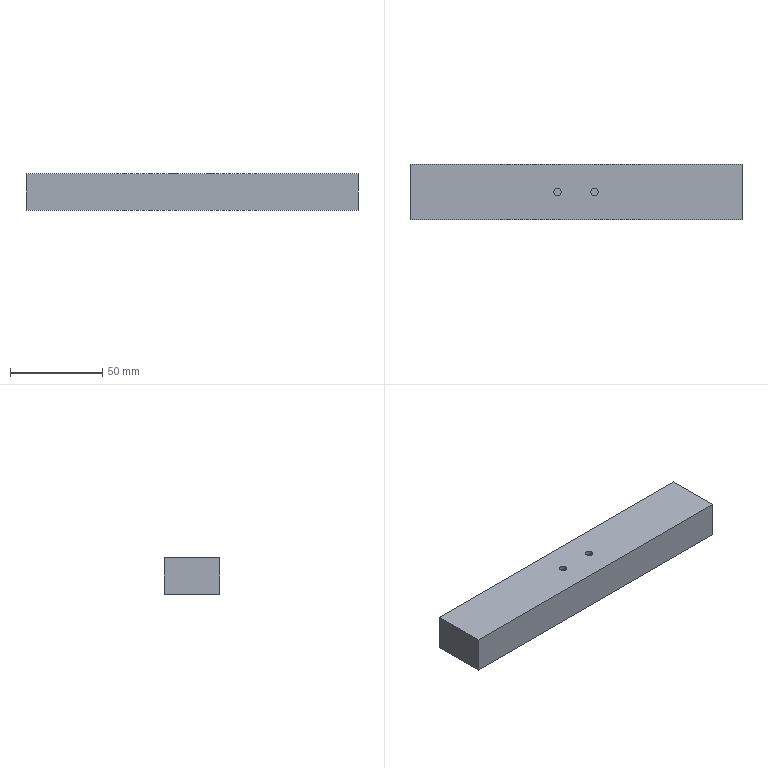Part | SolidWorks | features Extrusion 1, ICE 1 | 1 solid | 12 faces | box 180 x 30 x 20 mm | volume 107950 mm3 | plane 8 | cylinder 4 | commonest cylinder face diameters 4 x4
STEP:
#1=CARTESIAN_POINT('',(-12.,0.,18.));
#2=VERTEX_POINT('',#1);
#3=CARTESIAN_POINT('',(-8.,0.,18.));
#4=VERTEX_POINT('',#3);
#5=CARTESIAN_POINT('',(-10.,0.,18.));
#6=DIRECTION('',(0.,0.,1.));
#7=DIRECTION('',(1.,0.,0.));
#8=AXIS2_PLACEMENT_3D('',#5,#6,#7);
#9=CIRCLE('',#8,2.);
#10=EDGE_CURVE('',#2,#4,#9,.T.);
#11=ORIENTED_EDGE('',*,*,#10,.F.);
#12=CARTESIAN_POINT('',(-12.,0.,20.));
#13=VERTEX_POINT('',#12);
#14=CARTESIAN_POINT('',(-12.,0.,18.));
#15=DIRECTION('',(0.,0.,1.));
#16=VECTOR('',#15,1000.);
#17=LINE('',#14,#16);
#18=EDGE_CURVE('',#2,#13,#17,.T.);
#19=ORIENTED_EDGE('',*,*,#18,.T.);
#20=CARTESIAN_POINT('',(-8.,0.,20.));
#21=VERTEX_POINT('',#20);
#22=CARTESIAN_POINT('',(-10.,0.,20.));
#23=DIRECTION('',(0.,0.,1.));
#24=DIRECTION('',(1.,0.,0.));
#25=AXIS2_PLACEMENT_3D('',#22,#23,#24);
#26=CIRCLE('',#25,2.);
#27=EDGE_CURVE('',#13,#21,#26,.T.);
#28=ORIENTED_EDGE('',*,*,#27,.T.);
#29=CARTESIAN_POINT('',(-8.,0.,18.));
#30=DIRECTION('',(0.,0.,1.));
#31=VECTOR('',#30,1000.);
#32=LINE('',#29,#31);
#33=EDGE_CURVE('',#4,#21,#32,.T.);
#34=ORIENTED_EDGE('',*,*,#33,.F.);
#35=EDGE_LOOP('',(#11,#19,#28,#34));
#36=FACE_OUTER_BOUND('',#35,.T.);
#37=CARTESIAN_POINT('',(-10.,0.,18.));
#38=DIRECTION('',(0.,0.,1.));
#39=DIRECTION('',(1.,0.,0.));
#40=AXIS2_PLACEMENT_3D('',#37,#38,#39);
#41=CYLINDRICAL_SURFACE('',#40,2.);
#42=ADVANCED_FACE('',(#36),#41,.F.);
#43=CARTESIAN_POINT('',(8.,0.,18.));
#44=VERTEX_POINT('',#43);
#45=CARTESIAN_POINT('',(12.,0.,18.));
#46=VERTEX_POINT('',#45);
#47=CARTESIAN_POINT('',(10.,0.,18.));
#48=DIRECTION('',(0.,0.,1.));
#49=DIRECTION('',(1.,0.,0.));
#50=AXIS2_PLACEMENT_3D('',#47,#48,#49);
#51=CIRCLE('',#50,2.);
#52=EDGE_CURVE('',#44,#46,#51,.T.);
#53=ORIENTED_EDGE('',*,*,#52,.F.);
#54=CARTESIAN_POINT('',(8.,0.,20.));
#55=VERTEX_POINT('',#54);
#56=CARTESIAN_POINT('',(8.,0.,18.));
#57=DIRECTION('',(0.,0.,1.));
#58=VECTOR('',#57,1000.);
#59=LINE('',#56,#58);
#60=EDGE_CURVE('',#44,#55,#59,.T.);
#61=ORIENTED_EDGE('',*,*,#60,.T.);
#62=CARTESIAN_POINT('',(12.,0.,20.));
#63=VERTEX_POINT('',#62);
#64=CARTESIAN_POINT('',(10.,0.,20.));
#65=DIRECTION('',(0.,0.,1.));
#66=DIRECTION('',(1.,0.,0.));
#67=AXIS2_PLACEMENT_3D('',#64,#65,#66);
#68=CIRCLE('',#67,2.);
#69=EDGE_CURVE('',#55,#63,#68,.T.);
#70=ORIENTED_EDGE('',*,*,#69,.T.);
#71=CARTESIAN_POINT('',(12.,0.,18.));
#72=DIRECTION('',(0.,0.,1.));
#73=VECTOR('',#72,1000.);
#74=LINE('',#71,#73);
#75=EDGE_CURVE('',#46,#63,#74,.T.);
#76=ORIENTED_EDGE('',*,*,#75,.F.);
#77=EDGE_LOOP('',(#53,#61,#70,#76));
#78=FACE_OUTER_BOUND('',#77,.T.);
#79=CARTESIAN_POINT('',(10.,0.,18.));
#80=DIRECTION('',(0.,0.,1.));
#81=DIRECTION('',(1.,0.,0.));
#82=AXIS2_PLACEMENT_3D('',#79,#80,#81);
#83=CYLINDRICAL_SURFACE('',#82,2.);
#84=ADVANCED_FACE('',(#78),#83,.F.);
#85=CARTESIAN_POINT('',(-90.,15.,0.));
#86=VERTEX_POINT('',#85);
#87=CARTESIAN_POINT('',(-90.,-15.,0.));
#88=VERTEX_POINT('',#87);
#89=CARTESIAN_POINT('',(-90.,-15.,0.));
#90=DIRECTION('',(0.,-1.,0.));
#91=VECTOR('',#90,1000.);
#92=LINE('',#89,#91);
#93=EDGE_CURVE('',#86,#88,#92,.T.);
#94=ORIENTED_EDGE('',*,*,#93,.T.);
#95=CARTESIAN_POINT('',(-90.,-15.,20.));
#96=VERTEX_POINT('',#95);
#97=CARTESIAN_POINT('',(-90.,-15.,20.));
#98=DIRECTION('',(0.,0.,-1.));
#99=VECTOR('',#98,1000.);
#100=LINE('',#97,#99);
#101=EDGE_CURVE('',#96,#88,#100,.T.);
#102=ORIENTED_EDGE('',*,*,#101,.F.);
#103=CARTESIAN_POINT('',(-90.,15.,20.));
#104=VERTEX_POINT('',#103);
#105=CARTESIAN_POINT('',(-90.,-15.,20.));
#106=DIRECTION('',(0.,-1.,0.));
#107=VECTOR('',#106,1000.);
#108=LINE('',#105,#107);
#109=EDGE_CURVE('',#104,#96,#108,.T.);
#110=ORIENTED_EDGE('',*,*,#109,.F.);
#111=CARTESIAN_POINT('',(-90.,15.,20.));
#112=DIRECTION('',(0.,0.,-1.));
#113=VECTOR('',#112,1000.);
#114=LINE('',#111,#113);
#115=EDGE_CURVE('',#104,#86,#114,.T.);
#116=ORIENTED_EDGE('',*,*,#115,.T.);
#117=EDGE_LOOP('',(#94,#102,#110,#116));
#118=FACE_OUTER_BOUND('',#117,.T.);
#119=CARTESIAN_POINT('',(-90.,-15.,20.));
#120=DIRECTION('',(1.,0.,0.));
#121=DIRECTION('',(0.,0.,-1.));
#122=AXIS2_PLACEMENT_3D('',#119,#120,#121);
#123=PLANE('',#122);
#124=ADVANCED_FACE('',(#118),#123,.F.);
#125=CARTESIAN_POINT('',(90.,-15.,0.));
#126=VERTEX_POINT('',#125);
#127=CARTESIAN_POINT('',(90.,-15.,0.));
#128=DIRECTION('',(1.,0.,0.));
#129=VECTOR('',#128,1000.);
#130=LINE('',#127,#129);
#131=EDGE_CURVE('',#88,#126,#130,.T.);
#132=ORIENTED_EDGE('',*,*,#131,.T.);
#133=CARTESIAN_POINT('',(90.,-15.,20.));
#134=VERTEX_POINT('',#133);
#135=CARTESIAN_POINT('',(90.,-15.,20.));
#136=DIRECTION('',(0.,0.,-1.));
#137=VECTOR('',#136,1000.);
#138=LINE('',#135,#137);
#139=EDGE_CURVE('',#134,#126,#138,.T.);
#140=ORIENTED_EDGE('',*,*,#139,.F.);
#141=CARTESIAN_POINT('',(90.,-15.,20.));
#142=DIRECTION('',(1.,0.,0.));
#143=VECTOR('',#142,1000.);
#144=LINE('',#141,#143);
#145=EDGE_CURVE('',#96,#134,#144,.T.);
#146=ORIENTED_EDGE('',*,*,#145,.F.);
#147=ORIENTED_EDGE('',*,*,#101,.T.);
#148=EDGE_LOOP('',(#132,#140,#146,#147));
#149=FACE_OUTER_BOUND('',#148,.T.);
#150=CARTESIAN_POINT('',(90.,-15.,20.));
#151=DIRECTION('',(0.,1.,0.));
#152=DIRECTION('',(-1.,0.,0.));
#153=AXIS2_PLACEMENT_3D('',#150,#151,#152);
#154=PLANE('',#153);
#155=ADVANCED_FACE('',(#149),#154,.F.);
#156=CARTESIAN_POINT('',(90.,15.,0.));
#157=VERTEX_POINT('',#156);
#158=CARTESIAN_POINT('',(90.,-15.,0.));
#159=DIRECTION('',(0.,1.,0.));
#160=VECTOR('',#159,1000.);
#161=LINE('',#158,#160);
#162=EDGE_CURVE('',#126,#157,#161,.T.);
#163=ORIENTED_EDGE('',*,*,#162,.T.);
#164=CARTESIAN_POINT('',(90.,15.,20.));
#165=VERTEX_POINT('',#164);
#166=CARTESIAN_POINT('',(90.,15.,20.));
#167=DIRECTION('',(0.,0.,-1.));
#168=VECTOR('',#167,1000.);
#169=LINE('',#166,#168);
#170=EDGE_CURVE('',#165,#157,#169,.T.);
#171=ORIENTED_EDGE('',*,*,#170,.F.);
#172=CARTESIAN_POINT('',(90.,-15.,20.));
#173=DIRECTION('',(0.,1.,0.));
#174=VECTOR('',#173,1000.);
#175=LINE('',#172,#174);
#176=EDGE_CURVE('',#134,#165,#175,.T.);
#177=ORIENTED_EDGE('',*,*,#176,.F.);
#178=ORIENTED_EDGE('',*,*,#139,.T.);
#179=EDGE_LOOP('',(#163,#171,#177,#178));
#180=FACE_OUTER_BOUND('',#179,.T.);
#181=CARTESIAN_POINT('',(90.,-15.,20.));
#182=DIRECTION('',(-1.,0.,0.));
#183=DIRECTION('',(0.,0.,1.));
#184=AXIS2_PLACEMENT_3D('',#181,#182,#183);
#185=PLANE('',#184);
#186=ADVANCED_FACE('',(#180),#185,.F.);
#187=CARTESIAN_POINT('',(90.,15.,0.));
#188=DIRECTION('',(-1.,0.,0.));
#189=VECTOR('',#188,1000.);
#190=LINE('',#187,#189);
#191=EDGE_CURVE('',#157,#86,#190,.T.);
#192=ORIENTED_EDGE('',*,*,#191,.T.);
#193=ORIENTED_EDGE('',*,*,#115,.F.);
#194=CARTESIAN_POINT('',(90.,15.,20.));
#195=DIRECTION('',(-1.,0.,0.));
#196=VECTOR('',#195,1000.);
#197=LINE('',#194,#196);
#198=EDGE_CURVE('',#165,#104,#197,.T.);
#199=ORIENTED_EDGE('',*,*,#198,.F.);
#200=ORIENTED_EDGE('',*,*,#170,.T.);
#201=EDGE_LOOP('',(#192,#193,#199,#200));
#202=FACE_OUTER_BOUND('',#201,.T.);
#203=CARTESIAN_POINT('',(90.,15.,20.));
#204=DIRECTION('',(0.,-1.,0.));
#205=DIRECTION('',(1.,0.,0.));
#206=AXIS2_PLACEMENT_3D('',#203,#204,#205);
#207=PLANE('',#206);
#208=ADVANCED_FACE('',(#202),#207,.F.);
#209=CARTESIAN_POINT('',(-10.,0.,20.));
#210=DIRECTION('',(0.,0.,1.));
#211=DIRECTION('',(1.,0.,0.));
#212=AXIS2_PLACEMENT_3D('',#209,#210,#211);
#213=CIRCLE('',#212,2.);
#214=EDGE_CURVE('',#21,#13,#213,.T.);
#215=ORIENTED_EDGE('',*,*,#214,.F.);
#216=ORIENTED_EDGE('',*,*,#27,.F.);
#217=EDGE_LOOP('',(#215,#216));
#218=FACE_BOUND('',#217,.T.);
#219=CARTESIAN_POINT('',(10.,0.,20.));
#220=DIRECTION('',(0.,0.,1.));
#221=DIRECTION('',(1.,0.,0.));
#222=AXIS2_PLACEMENT_3D('',#219,#220,#221);
#223=CIRCLE('',#222,2.);
#224=EDGE_CURVE('',#63,#55,#223,.T.);
#225=ORIENTED_EDGE('',*,*,#224,.F.);
#226=ORIENTED_EDGE('',*,*,#69,.F.);
#227=EDGE_LOOP('',(#225,#226));
#228=FACE_BOUND('',#227,.T.);
#229=ORIENTED_EDGE('',*,*,#109,.T.);
#230=ORIENTED_EDGE('',*,*,#145,.T.);
#231=ORIENTED_EDGE('',*,*,#176,.T.);
#232=ORIENTED_EDGE('',*,*,#198,.T.);
#233=EDGE_LOOP('',(#229,#230,#231,#232));
#234=FACE_OUTER_BOUND('',#233,.T.);
#235=CARTESIAN_POINT('',(0.,0.,20.));
#236=DIRECTION('',(0.,0.,1.));
#237=DIRECTION('',(1.,0.,0.));
#238=AXIS2_PLACEMENT_3D('',#235,#236,#237);
#239=PLANE('',#238);
#240=ADVANCED_FACE('',(#218,#228,#234),#239,.T.);
#241=ORIENTED_EDGE('',*,*,#93,.F.);
#242=ORIENTED_EDGE('',*,*,#191,.F.);
#243=ORIENTED_EDGE('',*,*,#162,.F.);
#244=ORIENTED_EDGE('',*,*,#131,.F.);
#245=EDGE_LOOP('',(#241,#242,#243,#244));
#246=FACE_OUTER_BOUND('',#245,.T.);
#247=CARTESIAN_POINT('',(0.,0.,0.));
#248=DIRECTION('',(0.,0.,1.));
#249=DIRECTION('',(1.,0.,0.));
#250=AXIS2_PLACEMENT_3D('',#247,#248,#249);
#251=PLANE('',#250);
#252=ADVANCED_FACE('',(#246),#251,.F.);
#253=ORIENTED_EDGE('',*,*,#60,.F.);
#254=CARTESIAN_POINT('',(10.,0.,18.));
#255=DIRECTION('',(0.,0.,1.));
#256=DIRECTION('',(1.,0.,0.));
#257=AXIS2_PLACEMENT_3D('',#254,#255,#256);
#258=CIRCLE('',#257,2.);
#259=EDGE_CURVE('',#46,#44,#258,.T.);
#260=ORIENTED_EDGE('',*,*,#259,.F.);
#261=ORIENTED_EDGE('',*,*,#75,.T.);
#262=ORIENTED_EDGE('',*,*,#224,.T.);
#263=EDGE_LOOP('',(#253,#260,#261,#262));
#264=FACE_OUTER_BOUND('',#263,.T.);
#265=CARTESIAN_POINT('',(10.,0.,18.));
#266=DIRECTION('',(0.,0.,1.));
#267=DIRECTION('',(1.,0.,0.));
#268=AXIS2_PLACEMENT_3D('',#265,#266,#267);
#269=CYLINDRICAL_SURFACE('',#268,2.);
#270=ADVANCED_FACE('',(#264),#269,.F.);
#271=ORIENTED_EDGE('',*,*,#259,.T.);
#272=ORIENTED_EDGE('',*,*,#52,.T.);
#273=EDGE_LOOP('',(#271,#272));
#274=FACE_OUTER_BOUND('',#273,.T.);
#275=CARTESIAN_POINT('',(10.,0.,18.));
#276=DIRECTION('',(0.,0.,1.));
#277=DIRECTION('',(1.,0.,0.));
#278=AXIS2_PLACEMENT_3D('',#275,#276,#277);
#279=PLANE('',#278);
#280=ADVANCED_FACE('',(#274),#279,.T.);
#281=ORIENTED_EDGE('',*,*,#18,.F.);
#282=CARTESIAN_POINT('',(-10.,0.,18.));
#283=DIRECTION('',(0.,0.,1.));
#284=DIRECTION('',(1.,0.,0.));
#285=AXIS2_PLACEMENT_3D('',#282,#283,#284);
#286=CIRCLE('',#285,2.);
#287=EDGE_CURVE('',#4,#2,#286,.T.);
#288=ORIENTED_EDGE('',*,*,#287,.F.);
#289=ORIENTED_EDGE('',*,*,#33,.T.);
#290=ORIENTED_EDGE('',*,*,#214,.T.);
#291=EDGE_LOOP('',(#281,#288,#289,#290));
#292=FACE_OUTER_BOUND('',#291,.T.);
#293=CARTESIAN_POINT('',(-10.,0.,18.));
#294=DIRECTION('',(0.,0.,1.));
#295=DIRECTION('',(1.,0.,0.));
#296=AXIS2_PLACEMENT_3D('',#293,#294,#295);
#297=CYLINDRICAL_SURFACE('',#296,2.);
#298=ADVANCED_FACE('',(#292),#297,.F.);
#299=ORIENTED_EDGE('',*,*,#287,.T.);
#300=ORIENTED_EDGE('',*,*,#10,.T.);
#301=EDGE_LOOP('',(#299,#300));
#302=FACE_OUTER_BOUND('',#301,.T.);
#303=CARTESIAN_POINT('',(-10.,0.,18.));
#304=DIRECTION('',(0.,0.,1.));
#305=DIRECTION('',(1.,0.,0.));
#306=AXIS2_PLACEMENT_3D('',#303,#304,#305);
#307=PLANE('',#306);
#308=ADVANCED_FACE('',(#302),#307,.T.);
#309=CLOSED_SHELL('',(#42,#84,#124,#155,#186,#208,#240,#252,#270,#280,#298,#308));
#310=MANIFOLD_SOLID_BREP('',#309);
#311=CARTESIAN_POINT('',(0.,0.,0.));
#312=DIRECTION('',(0.,0.,1.));
#313=DIRECTION('',(1.,0.,0.));
#314=AXIS2_PLACEMENT_3D('',#311,#312,#313);
#315=(LENGTH_UNIT()NAMED_UNIT(*)SI_UNIT(.MILLI.,.METRE.));
#316=UNCERTAINTY_MEASURE_WITH_UNIT(LENGTH_MEASURE(0.00001),#315,'','');
#317=(NAMED_UNIT(*)PLANE_ANGLE_UNIT()SI_UNIT($,.RADIAN.));
#318=(NAMED_UNIT(*)SI_UNIT($,.STERADIAN.)SOLID_ANGLE_UNIT());
#319=(GEOMETRIC_REPRESENTATION_CONTEXT(3)GLOBAL_UNCERTAINTY_ASSIGNED_CONTEXT((#316))GLOBAL_UNIT_ASSIGNED_CONTEXT((#315,#317,#318))REPRESENTATION_CONTEXT('',''));
#320=ADVANCED_BREP_SHAPE_REPRESENTATION('',(#310,#314),#319);